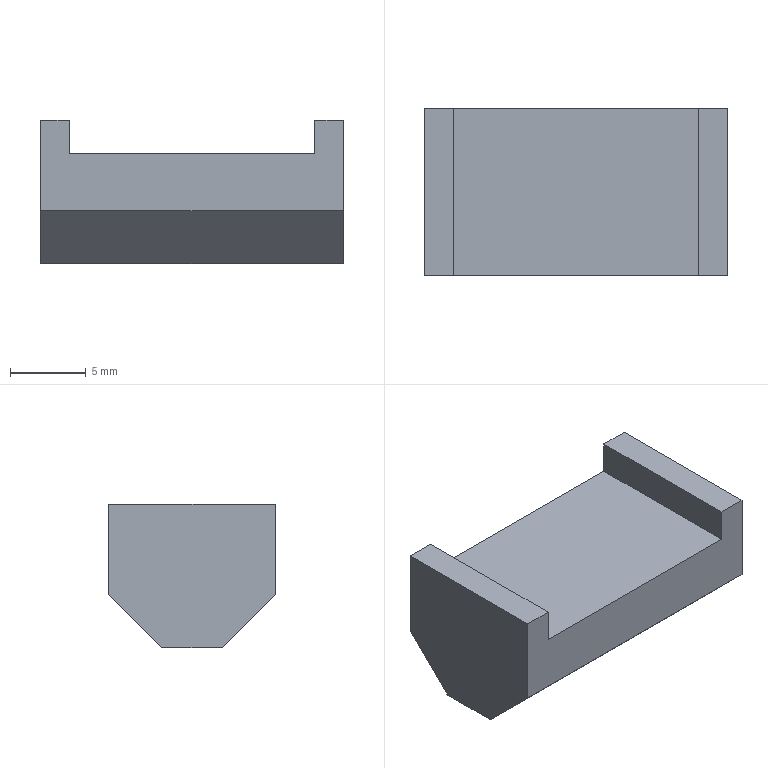Part | SolidWorks | features ICE 2, Extrusion 1, MirrorPattern 1 | 1 solid | 12 faces | box 20 x 11 x 9.5 mm | volume 1453 mm3 | plane 12
STEP:
#1=CARTESIAN_POINT('',(-10.,-2.,0.));
#2=VERTEX_POINT('',#1);
#3=CARTESIAN_POINT('',(-10.,-5.5,3.5));
#4=VERTEX_POINT('',#3);
#5=CARTESIAN_POINT('',(-10.,-5.5,3.5));
#6=DIRECTION('',(0.,-0.7071,0.7071));
#7=VECTOR('',#6,1000.);
#8=LINE('',#5,#7);
#9=EDGE_CURVE('',#2,#4,#8,.T.);
#10=ORIENTED_EDGE('',*,*,#9,.T.);
#11=CARTESIAN_POINT('',(-10.,-5.5,9.5));
#12=VERTEX_POINT('',#11);
#13=CARTESIAN_POINT('',(-10.,-5.5,9.5));
#14=DIRECTION('',(0.,0.,-1.));
#15=VECTOR('',#14,1000.);
#16=LINE('',#13,#15);
#17=EDGE_CURVE('',#12,#4,#16,.T.);
#18=ORIENTED_EDGE('',*,*,#17,.F.);
#19=CARTESIAN_POINT('',(-10.,5.5,9.5));
#20=VERTEX_POINT('',#19);
#21=CARTESIAN_POINT('',(-10.,5.5,9.5));
#22=DIRECTION('',(0.,-1.,0.));
#23=VECTOR('',#22,1000.);
#24=LINE('',#21,#23);
#25=EDGE_CURVE('',#20,#12,#24,.T.);
#26=ORIENTED_EDGE('',*,*,#25,.F.);
#27=CARTESIAN_POINT('',(-10.,5.5,3.5));
#28=VERTEX_POINT('',#27);
#29=CARTESIAN_POINT('',(-10.,5.5,9.5));
#30=DIRECTION('',(0.,0.,-1.));
#31=VECTOR('',#30,1000.);
#32=LINE('',#29,#31);
#33=EDGE_CURVE('',#20,#28,#32,.T.);
#34=ORIENTED_EDGE('',*,*,#33,.T.);
#35=CARTESIAN_POINT('',(-10.,2.,0.));
#36=VERTEX_POINT('',#35);
#37=CARTESIAN_POINT('',(-10.,5.5,3.5));
#38=DIRECTION('',(0.,0.7071,0.7071));
#39=VECTOR('',#38,1000.);
#40=LINE('',#37,#39);
#41=EDGE_CURVE('',#36,#28,#40,.T.);
#42=ORIENTED_EDGE('',*,*,#41,.F.);
#43=CARTESIAN_POINT('',(-10.,5.5,0.));
#44=DIRECTION('',(0.,-1.,0.));
#45=VECTOR('',#44,1000.);
#46=LINE('',#43,#45);
#47=EDGE_CURVE('',#36,#2,#46,.T.);
#48=ORIENTED_EDGE('',*,*,#47,.T.);
#49=EDGE_LOOP('',(#10,#18,#26,#34,#42,#48));
#50=FACE_OUTER_BOUND('',#49,.T.);
#51=CARTESIAN_POINT('',(-10.,5.5,9.5));
#52=DIRECTION('',(1.,0.,0.));
#53=DIRECTION('',(0.,0.,-1.));
#54=AXIS2_PLACEMENT_3D('',#51,#52,#53);
#55=PLANE('',#54);
#56=ADVANCED_FACE('',(#50),#55,.F.);
#57=CARTESIAN_POINT('',(10.,-5.5,3.5));
#58=VERTEX_POINT('',#57);
#59=CARTESIAN_POINT('',(10.,-5.5,3.5));
#60=DIRECTION('',(-1.,0.,0.));
#61=VECTOR('',#60,1000.);
#62=LINE('',#59,#61);
#63=EDGE_CURVE('',#58,#4,#62,.T.);
#64=ORIENTED_EDGE('',*,*,#63,.F.);
#65=CARTESIAN_POINT('',(10.,-5.5,9.5));
#66=VERTEX_POINT('',#65);
#67=CARTESIAN_POINT('',(10.,-5.5,9.5));
#68=DIRECTION('',(0.,0.,-1.));
#69=VECTOR('',#68,1000.);
#70=LINE('',#67,#69);
#71=EDGE_CURVE('',#66,#58,#70,.T.);
#72=ORIENTED_EDGE('',*,*,#71,.F.);
#73=CARTESIAN_POINT('',(8.1,-5.5,9.5));
#74=VERTEX_POINT('',#73);
#75=CARTESIAN_POINT('',(-10.,-5.5,9.5));
#76=DIRECTION('',(1.,0.,0.));
#77=VECTOR('',#76,1000.);
#78=LINE('',#75,#77);
#79=EDGE_CURVE('',#74,#66,#78,.T.);
#80=ORIENTED_EDGE('',*,*,#79,.F.);
#81=CARTESIAN_POINT('',(8.1,-5.5,7.3));
#82=VERTEX_POINT('',#81);
#83=CARTESIAN_POINT('',(8.1,-5.5,9.5));
#84=DIRECTION('',(0.,0.,-1.));
#85=VECTOR('',#84,1000.);
#86=LINE('',#83,#85);
#87=EDGE_CURVE('',#74,#82,#86,.T.);
#88=ORIENTED_EDGE('',*,*,#87,.T.);
#89=CARTESIAN_POINT('',(-8.1,-5.5,7.3));
#90=VERTEX_POINT('',#89);
#91=CARTESIAN_POINT('',(-10.,-5.5,7.3));
#92=DIRECTION('',(1.,0.,0.));
#93=VECTOR('',#92,1000.);
#94=LINE('',#91,#93);
#95=EDGE_CURVE('',#90,#82,#94,.T.);
#96=ORIENTED_EDGE('',*,*,#95,.F.);
#97=CARTESIAN_POINT('',(-8.1,-5.5,9.5));
#98=VERTEX_POINT('',#97);
#99=CARTESIAN_POINT('',(-8.1,-5.5,9.5));
#100=DIRECTION('',(0.,0.,1.));
#101=VECTOR('',#100,1000.);
#102=LINE('',#99,#101);
#103=EDGE_CURVE('',#90,#98,#102,.T.);
#104=ORIENTED_EDGE('',*,*,#103,.T.);
#105=CARTESIAN_POINT('',(-10.,-5.5,9.5));
#106=DIRECTION('',(1.,0.,0.));
#107=VECTOR('',#106,1000.);
#108=LINE('',#105,#107);
#109=EDGE_CURVE('',#12,#98,#108,.T.);
#110=ORIENTED_EDGE('',*,*,#109,.F.);
#111=ORIENTED_EDGE('',*,*,#17,.T.);
#112=EDGE_LOOP('',(#64,#72,#80,#88,#96,#104,#110,#111));
#113=FACE_OUTER_BOUND('',#112,.T.);
#114=CARTESIAN_POINT('',(-10.,-5.5,9.5));
#115=DIRECTION('',(0.,1.,0.));
#116=DIRECTION('',(0.,0.,1.));
#117=AXIS2_PLACEMENT_3D('',#114,#115,#116);
#118=PLANE('',#117);
#119=ADVANCED_FACE('',(#113),#118,.F.);
#120=CARTESIAN_POINT('',(10.,-2.,0.));
#121=VERTEX_POINT('',#120);
#122=CARTESIAN_POINT('',(10.,-5.5,3.5));
#123=DIRECTION('',(0.,-0.7071,0.7071));
#124=VECTOR('',#123,1000.);
#125=LINE('',#122,#124);
#126=EDGE_CURVE('',#121,#58,#125,.T.);
#127=ORIENTED_EDGE('',*,*,#126,.F.);
#128=CARTESIAN_POINT('',(10.,2.,0.));
#129=VERTEX_POINT('',#128);
#130=CARTESIAN_POINT('',(10.,5.5,0.));
#131=DIRECTION('',(0.,1.,0.));
#132=VECTOR('',#131,1000.);
#133=LINE('',#130,#132);
#134=EDGE_CURVE('',#121,#129,#133,.T.);
#135=ORIENTED_EDGE('',*,*,#134,.T.);
#136=CARTESIAN_POINT('',(10.,5.5,3.5));
#137=VERTEX_POINT('',#136);
#138=CARTESIAN_POINT('',(10.,5.5,3.5));
#139=DIRECTION('',(0.,0.7071,0.7071));
#140=VECTOR('',#139,1000.);
#141=LINE('',#138,#140);
#142=EDGE_CURVE('',#129,#137,#141,.T.);
#143=ORIENTED_EDGE('',*,*,#142,.T.);
#144=CARTESIAN_POINT('',(10.,5.5,9.5));
#145=VERTEX_POINT('',#144);
#146=CARTESIAN_POINT('',(10.,5.5,9.5));
#147=DIRECTION('',(0.,0.,-1.));
#148=VECTOR('',#147,1000.);
#149=LINE('',#146,#148);
#150=EDGE_CURVE('',#145,#137,#149,.T.);
#151=ORIENTED_EDGE('',*,*,#150,.F.);
#152=CARTESIAN_POINT('',(10.,5.5,9.5));
#153=DIRECTION('',(0.,1.,0.));
#154=VECTOR('',#153,1000.);
#155=LINE('',#152,#154);
#156=EDGE_CURVE('',#66,#145,#155,.T.);
#157=ORIENTED_EDGE('',*,*,#156,.F.);
#158=ORIENTED_EDGE('',*,*,#71,.T.);
#159=EDGE_LOOP('',(#127,#135,#143,#151,#157,#158));
#160=FACE_OUTER_BOUND('',#159,.T.);
#161=CARTESIAN_POINT('',(10.,5.5,9.5));
#162=DIRECTION('',(-1.,0.,0.));
#163=DIRECTION('',(0.,0.,1.));
#164=AXIS2_PLACEMENT_3D('',#161,#162,#163);
#165=PLANE('',#164);
#166=ADVANCED_FACE('',(#160),#165,.F.);
#167=CARTESIAN_POINT('',(10.,-2.,0.));
#168=DIRECTION('',(-1.,0.,0.));
#169=VECTOR('',#168,1000.);
#170=LINE('',#167,#169);
#171=EDGE_CURVE('',#121,#2,#170,.T.);
#172=ORIENTED_EDGE('',*,*,#171,.T.);
#173=ORIENTED_EDGE('',*,*,#47,.F.);
#174=CARTESIAN_POINT('',(10.,2.,0.));
#175=DIRECTION('',(-1.,0.,0.));
#176=VECTOR('',#175,1000.);
#177=LINE('',#174,#176);
#178=EDGE_CURVE('',#129,#36,#177,.T.);
#179=ORIENTED_EDGE('',*,*,#178,.F.);
#180=ORIENTED_EDGE('',*,*,#134,.F.);
#181=EDGE_LOOP('',(#172,#173,#179,#180));
#182=FACE_OUTER_BOUND('',#181,.T.);
#183=CARTESIAN_POINT('',(0.,0.,0.));
#184=DIRECTION('',(0.,0.,1.));
#185=DIRECTION('',(1.,0.,0.));
#186=AXIS2_PLACEMENT_3D('',#183,#184,#185);
#187=PLANE('',#186);
#188=ADVANCED_FACE('',(#182),#187,.F.);
#189=CARTESIAN_POINT('',(-8.1,5.5,9.5));
#190=VERTEX_POINT('',#189);
#191=CARTESIAN_POINT('',(-8.1,0.,9.5));
#192=DIRECTION('',(0.,-1.,0.));
#193=VECTOR('',#192,1000.);
#194=LINE('',#191,#193);
#195=EDGE_CURVE('',#190,#98,#194,.T.);
#196=ORIENTED_EDGE('',*,*,#195,.F.);
#197=CARTESIAN_POINT('',(-10.,5.5,9.5));
#198=DIRECTION('',(-1.,0.,0.));
#199=VECTOR('',#198,1000.);
#200=LINE('',#197,#199);
#201=EDGE_CURVE('',#190,#20,#200,.T.);
#202=ORIENTED_EDGE('',*,*,#201,.T.);
#203=ORIENTED_EDGE('',*,*,#25,.T.);
#204=ORIENTED_EDGE('',*,*,#109,.T.);
#205=EDGE_LOOP('',(#196,#202,#203,#204));
#206=FACE_OUTER_BOUND('',#205,.T.);
#207=CARTESIAN_POINT('',(0.,0.,9.5));
#208=DIRECTION('',(0.,0.,1.));
#209=DIRECTION('',(1.,0.,0.));
#210=AXIS2_PLACEMENT_3D('',#207,#208,#209);
#211=PLANE('',#210);
#212=ADVANCED_FACE('',(#206),#211,.T.);
#213=ORIENTED_EDGE('',*,*,#150,.T.);
#214=CARTESIAN_POINT('',(10.,5.5,3.5));
#215=DIRECTION('',(-1.,0.,0.));
#216=VECTOR('',#215,1000.);
#217=LINE('',#214,#216);
#218=EDGE_CURVE('',#137,#28,#217,.T.);
#219=ORIENTED_EDGE('',*,*,#218,.T.);
#220=ORIENTED_EDGE('',*,*,#33,.F.);
#221=ORIENTED_EDGE('',*,*,#201,.F.);
#222=CARTESIAN_POINT('',(-8.1,5.5,7.3));
#223=VERTEX_POINT('',#222);
#224=CARTESIAN_POINT('',(-8.1,5.5,9.5));
#225=DIRECTION('',(0.,0.,-1.));
#226=VECTOR('',#225,1000.);
#227=LINE('',#224,#226);
#228=EDGE_CURVE('',#190,#223,#227,.T.);
#229=ORIENTED_EDGE('',*,*,#228,.T.);
#230=CARTESIAN_POINT('',(8.1,5.5,7.3));
#231=VERTEX_POINT('',#230);
#232=CARTESIAN_POINT('',(-10.,5.5,7.3));
#233=DIRECTION('',(-1.,0.,0.));
#234=VECTOR('',#233,1000.);
#235=LINE('',#232,#234);
#236=EDGE_CURVE('',#231,#223,#235,.T.);
#237=ORIENTED_EDGE('',*,*,#236,.F.);
#238=CARTESIAN_POINT('',(8.1,5.5,9.5));
#239=VERTEX_POINT('',#238);
#240=CARTESIAN_POINT('',(8.1,5.5,9.5));
#241=DIRECTION('',(0.,0.,1.));
#242=VECTOR('',#241,1000.);
#243=LINE('',#240,#242);
#244=EDGE_CURVE('',#231,#239,#243,.T.);
#245=ORIENTED_EDGE('',*,*,#244,.T.);
#246=CARTESIAN_POINT('',(-10.,5.5,9.5));
#247=DIRECTION('',(-1.,0.,0.));
#248=VECTOR('',#247,1000.);
#249=LINE('',#246,#248);
#250=EDGE_CURVE('',#145,#239,#249,.T.);
#251=ORIENTED_EDGE('',*,*,#250,.F.);
#252=EDGE_LOOP('',(#213,#219,#220,#221,#229,#237,#245,#251));
#253=FACE_OUTER_BOUND('',#252,.T.);
#254=CARTESIAN_POINT('',(-10.,5.5,9.5));
#255=DIRECTION('',(0.,-1.,0.));
#256=DIRECTION('',(0.,0.,-1.));
#257=AXIS2_PLACEMENT_3D('',#254,#255,#256);
#258=PLANE('',#257);
#259=ADVANCED_FACE('',(#253),#258,.F.);
#260=CARTESIAN_POINT('',(8.1,0.,9.5));
#261=DIRECTION('',(0.,1.,0.));
#262=VECTOR('',#261,1000.);
#263=LINE('',#260,#262);
#264=EDGE_CURVE('',#74,#239,#263,.T.);
#265=ORIENTED_EDGE('',*,*,#264,.F.);
#266=ORIENTED_EDGE('',*,*,#79,.T.);
#267=ORIENTED_EDGE('',*,*,#156,.T.);
#268=ORIENTED_EDGE('',*,*,#250,.T.);
#269=EDGE_LOOP('',(#265,#266,#267,#268));
#270=FACE_OUTER_BOUND('',#269,.T.);
#271=CARTESIAN_POINT('',(0.,0.,9.5));
#272=DIRECTION('',(0.,0.,1.));
#273=DIRECTION('',(1.,0.,0.));
#274=AXIS2_PLACEMENT_3D('',#271,#272,#273);
#275=PLANE('',#274);
#276=ADVANCED_FACE('',(#270),#275,.T.);
#277=ORIENTED_EDGE('',*,*,#95,.T.);
#278=CARTESIAN_POINT('',(8.1,14.948,7.3));
#279=DIRECTION('',(0.,1.,0.));
#280=VECTOR('',#279,1000.);
#281=LINE('',#278,#280);
#282=EDGE_CURVE('',#82,#231,#281,.T.);
#283=ORIENTED_EDGE('',*,*,#282,.T.);
#284=ORIENTED_EDGE('',*,*,#236,.T.);
#285=CARTESIAN_POINT('',(-8.1,14.948,7.3));
#286=DIRECTION('',(0.,-1.,0.));
#287=VECTOR('',#286,1000.);
#288=LINE('',#285,#287);
#289=EDGE_CURVE('',#223,#90,#288,.T.);
#290=ORIENTED_EDGE('',*,*,#289,.T.);
#291=EDGE_LOOP('',(#277,#283,#284,#290));
#292=FACE_OUTER_BOUND('',#291,.T.);
#293=CARTESIAN_POINT('',(0.,0.,7.3));
#294=DIRECTION('',(0.,0.,1.));
#295=DIRECTION('',(1.,0.,0.));
#296=AXIS2_PLACEMENT_3D('',#293,#294,#295);
#297=PLANE('',#296);
#298=ADVANCED_FACE('',(#292),#297,.T.);
#299=ORIENTED_EDGE('',*,*,#289,.F.);
#300=ORIENTED_EDGE('',*,*,#228,.F.);
#301=ORIENTED_EDGE('',*,*,#195,.T.);
#302=ORIENTED_EDGE('',*,*,#103,.F.);
#303=EDGE_LOOP('',(#299,#300,#301,#302));
#304=FACE_OUTER_BOUND('',#303,.T.);
#305=CARTESIAN_POINT('',(-8.1,14.948,7.3));
#306=DIRECTION('',(-1.,0.,0.));
#307=DIRECTION('',(0.,0.,1.));
#308=AXIS2_PLACEMENT_3D('',#305,#306,#307);
#309=PLANE('',#308);
#310=ADVANCED_FACE('',(#304),#309,.F.);
#311=ORIENTED_EDGE('',*,*,#264,.T.);
#312=ORIENTED_EDGE('',*,*,#244,.F.);
#313=ORIENTED_EDGE('',*,*,#282,.F.);
#314=ORIENTED_EDGE('',*,*,#87,.F.);
#315=EDGE_LOOP('',(#311,#312,#313,#314));
#316=FACE_OUTER_BOUND('',#315,.T.);
#317=CARTESIAN_POINT('',(8.1,14.948,7.3));
#318=DIRECTION('',(1.,0.,0.));
#319=DIRECTION('',(0.,0.,-1.));
#320=AXIS2_PLACEMENT_3D('',#317,#318,#319);
#321=PLANE('',#320);
#322=ADVANCED_FACE('',(#316),#321,.F.);
#323=ORIENTED_EDGE('',*,*,#41,.T.);
#324=ORIENTED_EDGE('',*,*,#218,.F.);
#325=ORIENTED_EDGE('',*,*,#142,.F.);
#326=ORIENTED_EDGE('',*,*,#178,.T.);
#327=EDGE_LOOP('',(#323,#324,#325,#326));
#328=FACE_OUTER_BOUND('',#327,.T.);
#329=CARTESIAN_POINT('',(10.,5.5,3.5));
#330=DIRECTION('',(0.,-0.7071,0.7071));
#331=DIRECTION('',(0.,-0.7071,-0.7071));
#332=AXIS2_PLACEMENT_3D('',#329,#330,#331);
#333=PLANE('',#332);
#334=ADVANCED_FACE('',(#328),#333,.F.);
#335=ORIENTED_EDGE('',*,*,#9,.F.);
#336=ORIENTED_EDGE('',*,*,#171,.F.);
#337=ORIENTED_EDGE('',*,*,#126,.T.);
#338=ORIENTED_EDGE('',*,*,#63,.T.);
#339=EDGE_LOOP('',(#335,#336,#337,#338));
#340=FACE_OUTER_BOUND('',#339,.T.);
#341=CARTESIAN_POINT('',(10.,-5.5,3.5));
#342=DIRECTION('',(0.,-0.7071,-0.7071));
#343=DIRECTION('',(0.,0.7071,-0.7071));
#344=AXIS2_PLACEMENT_3D('',#341,#342,#343);
#345=PLANE('',#344);
#346=ADVANCED_FACE('',(#340),#345,.T.);
#347=CLOSED_SHELL('',(#56,#119,#166,#188,#212,#259,#276,#298,#310,#322,#334,#346));
#348=MANIFOLD_SOLID_BREP('',#347);
#349=CARTESIAN_POINT('',(0.,0.,0.));
#350=DIRECTION('',(0.,0.,1.));
#351=DIRECTION('',(1.,0.,0.));
#352=AXIS2_PLACEMENT_3D('',#349,#350,#351);
#353=(LENGTH_UNIT()NAMED_UNIT(*)SI_UNIT(.MILLI.,.METRE.));
#354=UNCERTAINTY_MEASURE_WITH_UNIT(LENGTH_MEASURE(0.00001),#353,'','');
#355=(NAMED_UNIT(*)PLANE_ANGLE_UNIT()SI_UNIT($,.RADIAN.));
#356=(NAMED_UNIT(*)SI_UNIT($,.STERADIAN.)SOLID_ANGLE_UNIT());
#357=(GEOMETRIC_REPRESENTATION_CONTEXT(3)GLOBAL_UNCERTAINTY_ASSIGNED_CONTEXT((#354))GLOBAL_UNIT_ASSIGNED_CONTEXT((#353,#355,#356))REPRESENTATION_CONTEXT('',''));
#358=ADVANCED_BREP_SHAPE_REPRESENTATION('',(#348,#352),#357);